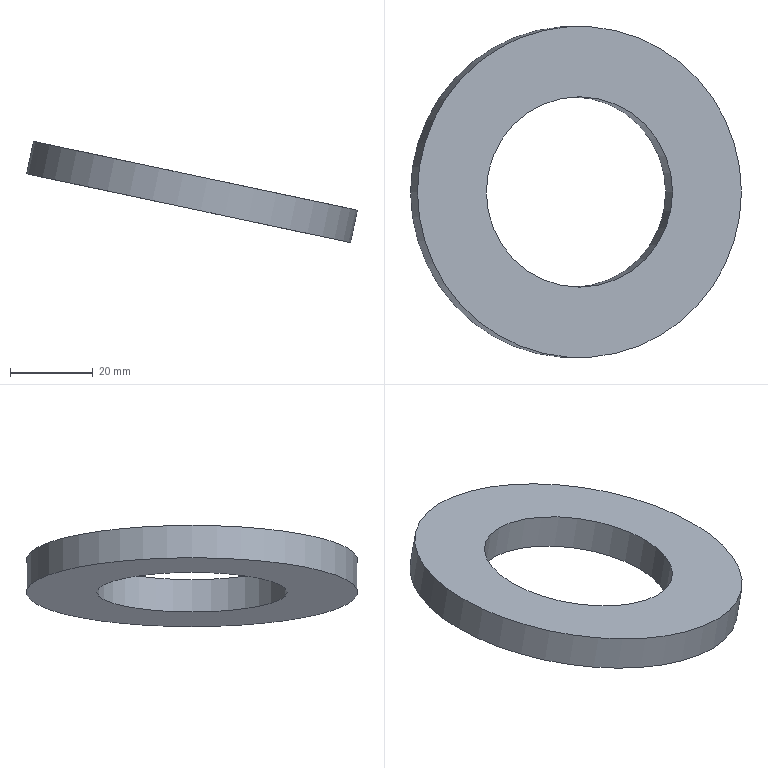Part | STEP file | HL4GZ-1.862.558 (flat washer GB_T 95 45) | 1 solid | 4 faces | box 79.915 x 80 x 24.458 mm | volume 26917 mm3 | plane 2 | cylinder 2 | commonest cylinder face diameters 46 x1 80 x1
STEP:
#1=CARTESIAN_POINT('',(0.,0.,0.));
#2=DIRECTION('',(0.,0.,1.));
#3=DIRECTION('',(1.,0.,0.));
#4=AXIS2_PLACEMENT_3D('',#1,#2,#3);
#5=CARTESIAN_POINT('',(1955.812,0.00003081,-342.814));
#6=VERTEX_POINT('',#5);
#7=CARTESIAN_POINT('',(1978.31,0.00003081,-347.596));
#8=DIRECTION('',(0.2079,0.,0.9781));
#9=DIRECTION('',(-0.9781,0.,0.2079));
#10=AXIS2_PLACEMENT_3D('',#7,#8,#9);
#11=CIRCLE('',#10,23.);
#12=CARTESIAN_POINT('',(1978.31,0.00003081,-347.596));
#13=DIRECTION('',(-0.2079,0.,-0.9781));
#14=DIRECTION('',(0.,-1.,0.));
#15=AXIS2_PLACEMENT_3D('',#12,#13,#14);
#16=PLANE('',#15);
#17=CARTESIAN_POINT('',(0.,23.));
#18=CARTESIAN_POINT('',(39.837,23.));
#19=CARTESIAN_POINT('',(19.919,-11.5));
#20=CARTESIAN_POINT('',(0.,-46.));
#21=CARTESIAN_POINT('',(-19.919,-11.5));
#22=CARTESIAN_POINT('',(-39.837,23.));
#23=CARTESIAN_POINT('',(0.,23.));
#24=(BOUNDED_CURVE()B_SPLINE_CURVE(2,(#17,#18,#19,#20,#21,#22,#23),.UNSPECIFIED.,.T.,.F.)B_SPLINE_CURVE_WITH_KNOTS((1,2,2,2,2,1),(-2.094,0.,2.094,4.189,6.283,8.378),.UNSPECIFIED.)CURVE()GEOMETRIC_REPRESENTATION_ITEM()RATIONAL_B_SPLINE_CURVE((1.,0.5,1.,0.5,1.,0.5,1.))REPRESENTATION_ITEM(''));
#25=(GEOMETRIC_REPRESENTATION_CONTEXT(2)PARAMETRIC_REPRESENTATION_CONTEXT()REPRESENTATION_CONTEXT('',''));
#26=DEFINITIONAL_REPRESENTATION('',(#24),#25);
#27=PCURVE('',#16,#26);
#28=CARTESIAN_POINT('',(1978.31,0.00003081,-347.596));
#29=DIRECTION('',(0.2079,0.,0.9781));
#30=DIRECTION('',(0.9781,0.,-0.2079));
#31=AXIS2_PLACEMENT_3D('',#28,#29,#30);
#32=CYLINDRICAL_SURFACE('',#31,23.);
#33=CARTESIAN_POINT('',(3.142,0.));
#34=DIRECTION('',(1.,0.));
#35=VECTOR('',#34,1.);
#36=LINE('',#33,#35);
#37=(GEOMETRIC_REPRESENTATION_CONTEXT(2)PARAMETRIC_REPRESENTATION_CONTEXT()REPRESENTATION_CONTEXT('',''));
#38=DEFINITIONAL_REPRESENTATION('',(#36),#37);
#39=PCURVE('',#32,#38);
#40=SURFACE_CURVE('',#11,(#27,#39),.PCURVE_S1.);
#41=EDGE_CURVE('',#6,#6,#40,.T.);
#42=ORIENTED_EDGE('',*,*,#41,.T.);
#43=EDGE_LOOP('',(#42));
#44=FACE_BOUND('',#43,.T.);
#45=CARTESIAN_POINT('',(1939.184,0.00003081,-339.28));
#46=VERTEX_POINT('',#45);
#47=CARTESIAN_POINT('',(1978.31,0.00003081,-347.596));
#48=DIRECTION('',(-0.2079,0.,-0.9781));
#49=DIRECTION('',(-0.9781,0.,0.2079));
#50=AXIS2_PLACEMENT_3D('',#47,#48,#49);
#51=CIRCLE('',#50,40.);
#52=CARTESIAN_POINT('',(0.,0.));
#53=DIRECTION('',(0.,1.));
#54=AXIS2_PLACEMENT_2D('',#52,#53);
#55=CIRCLE('',#54,40.);
#56=(GEOMETRIC_REPRESENTATION_CONTEXT(2)PARAMETRIC_REPRESENTATION_CONTEXT()REPRESENTATION_CONTEXT('',''));
#57=DEFINITIONAL_REPRESENTATION('',(#55),#56);
#58=PCURVE('',#16,#57);
#59=CARTESIAN_POINT('',(1978.31,0.00003081,-347.596));
#60=DIRECTION('',(0.2079,0.,0.9781));
#61=DIRECTION('',(0.9781,0.,-0.2079));
#62=AXIS2_PLACEMENT_3D('',#59,#60,#61);
#63=CYLINDRICAL_SURFACE('',#62,40.);
#64=CARTESIAN_POINT('',(9.425,0.));
#65=DIRECTION('',(-1.,0.));
#66=VECTOR('',#65,1.);
#67=LINE('',#64,#66);
#68=(GEOMETRIC_REPRESENTATION_CONTEXT(2)PARAMETRIC_REPRESENTATION_CONTEXT()REPRESENTATION_CONTEXT('',''));
#69=DEFINITIONAL_REPRESENTATION('',(#67),#68);
#70=PCURVE('',#63,#69);
#71=SURFACE_CURVE('',#51,(#58,#70),.PCURVE_S1.);
#72=EDGE_CURVE('',#46,#46,#71,.T.);
#73=ORIENTED_EDGE('',*,*,#72,.T.);
#74=EDGE_LOOP('',(#73));
#75=FACE_BOUND('',#74,.T.);
#76=ADVANCED_FACE('',(#44,#75),#16,.T.);
#77=CARTESIAN_POINT('',(1957.476,0.00003081,-334.989));
#78=VERTEX_POINT('',#77);
#79=CARTESIAN_POINT('',(1979.973,0.00003081,-339.771));
#80=DIRECTION('',(-0.2079,0.,-0.9781));
#81=DIRECTION('',(-0.9781,0.,0.2079));
#82=AXIS2_PLACEMENT_3D('',#79,#80,#81);
#83=CIRCLE('',#82,23.);
#84=CARTESIAN_POINT('',(1979.973,0.00003081,-339.771));
#85=DIRECTION('',(-0.2079,0.,-0.9781));
#86=DIRECTION('',(0.,-1.,0.));
#87=AXIS2_PLACEMENT_3D('',#84,#85,#86);
#88=PLANE('',#87);
#89=CARTESIAN_POINT('',(0.,0.));
#90=DIRECTION('',(0.,1.));
#91=AXIS2_PLACEMENT_2D('',#89,#90);
#92=CIRCLE('',#91,23.);
#93=(GEOMETRIC_REPRESENTATION_CONTEXT(2)PARAMETRIC_REPRESENTATION_CONTEXT()REPRESENTATION_CONTEXT('',''));
#94=DEFINITIONAL_REPRESENTATION('',(#92),#93);
#95=PCURVE('',#88,#94);
#96=CARTESIAN_POINT('',(9.425,8.));
#97=DIRECTION('',(-1.,0.));
#98=VECTOR('',#97,1.);
#99=LINE('',#96,#98);
#100=(GEOMETRIC_REPRESENTATION_CONTEXT(2)PARAMETRIC_REPRESENTATION_CONTEXT()REPRESENTATION_CONTEXT('',''));
#101=DEFINITIONAL_REPRESENTATION('',(#99),#100);
#102=PCURVE('',#32,#101);
#103=SURFACE_CURVE('',#83,(#95,#102),.PCURVE_S1.);
#104=EDGE_CURVE('',#78,#78,#103,.T.);
#105=ORIENTED_EDGE('',*,*,#104,.T.);
#106=EDGE_LOOP('',(#105));
#107=FACE_BOUND('',#106,.T.);
#108=CARTESIAN_POINT('',(1940.847,0.00003081,-331.455));
#109=VERTEX_POINT('',#108);
#110=CARTESIAN_POINT('',(1979.973,0.00003081,-339.771));
#111=DIRECTION('',(-0.2079,0.,-0.9781));
#112=DIRECTION('',(-0.9781,0.,0.2079));
#113=AXIS2_PLACEMENT_3D('',#110,#111,#112);
#114=CIRCLE('',#113,40.);
#115=CARTESIAN_POINT('',(0.,0.));
#116=DIRECTION('',(0.,1.));
#117=AXIS2_PLACEMENT_2D('',#115,#116);
#118=CIRCLE('',#117,40.);
#119=(GEOMETRIC_REPRESENTATION_CONTEXT(2)PARAMETRIC_REPRESENTATION_CONTEXT()REPRESENTATION_CONTEXT('',''));
#120=DEFINITIONAL_REPRESENTATION('',(#118),#119);
#121=PCURVE('',#88,#120);
#122=CARTESIAN_POINT('',(9.425,8.));
#123=DIRECTION('',(-1.,0.));
#124=VECTOR('',#123,1.);
#125=LINE('',#122,#124);
#126=(GEOMETRIC_REPRESENTATION_CONTEXT(2)PARAMETRIC_REPRESENTATION_CONTEXT()REPRESENTATION_CONTEXT('',''));
#127=DEFINITIONAL_REPRESENTATION('',(#125),#126);
#128=PCURVE('',#63,#127);
#129=SURFACE_CURVE('',#114,(#121,#128),.PCURVE_S1.);
#130=EDGE_CURVE('',#109,#109,#129,.T.);
#131=ORIENTED_EDGE('',*,*,#130,.F.);
#132=EDGE_LOOP('',(#131));
#133=FACE_BOUND('',#132,.T.);
#134=ADVANCED_FACE('',(#107,#133),#88,.F.);
#135=ORIENTED_EDGE('',*,*,#72,.F.);
#136=CARTESIAN_POINT('',(1939.184,0.00003081,-339.28));
#137=CARTESIAN_POINT('',(1940.847,0.00003081,-331.455));
#138=B_SPLINE_CURVE_WITH_KNOTS('',1,(#136,#137),.UNSPECIFIED.,.F.,.F.,(2,2),(0.,8.),.PIECEWISE_BEZIER_KNOTS.);
#139=CARTESIAN_POINT('',(9.425,0.));
#140=DIRECTION('',(0.,1.));
#141=VECTOR('',#140,1.);
#142=LINE('',#139,#141);
#143=(GEOMETRIC_REPRESENTATION_CONTEXT(2)PARAMETRIC_REPRESENTATION_CONTEXT()REPRESENTATION_CONTEXT('',''));
#144=DEFINITIONAL_REPRESENTATION('',(#142),#143);
#145=PCURVE('',#63,#144);
#146=CARTESIAN_POINT('',(3.142,0.));
#147=DIRECTION('',(0.,1.));
#148=VECTOR('',#147,1.);
#149=LINE('',#146,#148);
#150=(GEOMETRIC_REPRESENTATION_CONTEXT(2)PARAMETRIC_REPRESENTATION_CONTEXT()REPRESENTATION_CONTEXT('',''));
#151=DEFINITIONAL_REPRESENTATION('',(#149),#150);
#152=PCURVE('',#63,#151);
#153=SEAM_CURVE('',#138,(#145,#152),.PCURVE_S1.);
#154=EDGE_CURVE('',#46,#109,#153,.T.);
#155=ORIENTED_EDGE('',*,*,#154,.T.);
#156=ORIENTED_EDGE('',*,*,#130,.T.);
#157=ORIENTED_EDGE('',*,*,#154,.F.);
#158=EDGE_LOOP('',(#135,#155,#156,#157));
#159=FACE_BOUND('',#158,.T.);
#160=ADVANCED_FACE('',(#159),#63,.T.);
#161=ORIENTED_EDGE('',*,*,#41,.T.);
#162=CARTESIAN_POINT('',(1955.812,0.00003081,-342.814));
#163=CARTESIAN_POINT('',(1957.476,0.00003081,-334.989));
#164=B_SPLINE_CURVE_WITH_KNOTS('',1,(#162,#163),.UNSPECIFIED.,.F.,.F.,(2,2),(0.,8.),.PIECEWISE_BEZIER_KNOTS.);
#165=CARTESIAN_POINT('',(9.425,0.));
#166=DIRECTION('',(0.,1.));
#167=VECTOR('',#166,1.);
#168=LINE('',#165,#167);
#169=(GEOMETRIC_REPRESENTATION_CONTEXT(2)PARAMETRIC_REPRESENTATION_CONTEXT()REPRESENTATION_CONTEXT('',''));
#170=DEFINITIONAL_REPRESENTATION('',(#168),#169);
#171=PCURVE('',#32,#170);
#172=CARTESIAN_POINT('',(3.142,0.));
#173=DIRECTION('',(0.,1.));
#174=VECTOR('',#173,1.);
#175=LINE('',#172,#174);
#176=(GEOMETRIC_REPRESENTATION_CONTEXT(2)PARAMETRIC_REPRESENTATION_CONTEXT()REPRESENTATION_CONTEXT('',''));
#177=DEFINITIONAL_REPRESENTATION('',(#175),#176);
#178=PCURVE('',#32,#177);
#179=SEAM_CURVE('',#164,(#171,#178),.PCURVE_S1.);
#180=EDGE_CURVE('',#6,#78,#179,.T.);
#181=ORIENTED_EDGE('',*,*,#180,.T.);
#182=ORIENTED_EDGE('',*,*,#104,.T.);
#183=ORIENTED_EDGE('',*,*,#180,.F.);
#184=EDGE_LOOP('',(#161,#181,#182,#183));
#185=FACE_BOUND('',#184,.F.);
#186=ADVANCED_FACE('',(#185),#32,.F.);
#187=CLOSED_SHELL('',(#76,#134,#160,#186));
#188=MANIFOLD_SOLID_BREP('',#187);
#189=(LENGTH_UNIT()NAMED_UNIT(*)SI_UNIT(.MILLI.,.METRE.));
#190=UNCERTAINTY_MEASURE_WITH_UNIT(LENGTH_MEASURE(0.00001),#189,'','');
#191=(NAMED_UNIT(*)PLANE_ANGLE_UNIT()SI_UNIT($,.RADIAN.));
#192=(NAMED_UNIT(*)SI_UNIT($,.STERADIAN.)SOLID_ANGLE_UNIT());
#193=(GEOMETRIC_REPRESENTATION_CONTEXT(3)GLOBAL_UNCERTAINTY_ASSIGNED_CONTEXT((#190))GLOBAL_UNIT_ASSIGNED_CONTEXT((#189,#191,#192))REPRESENTATION_CONTEXT('',''));
#194=ADVANCED_BREP_SHAPE_REPRESENTATION('',(#4,#188),#193);